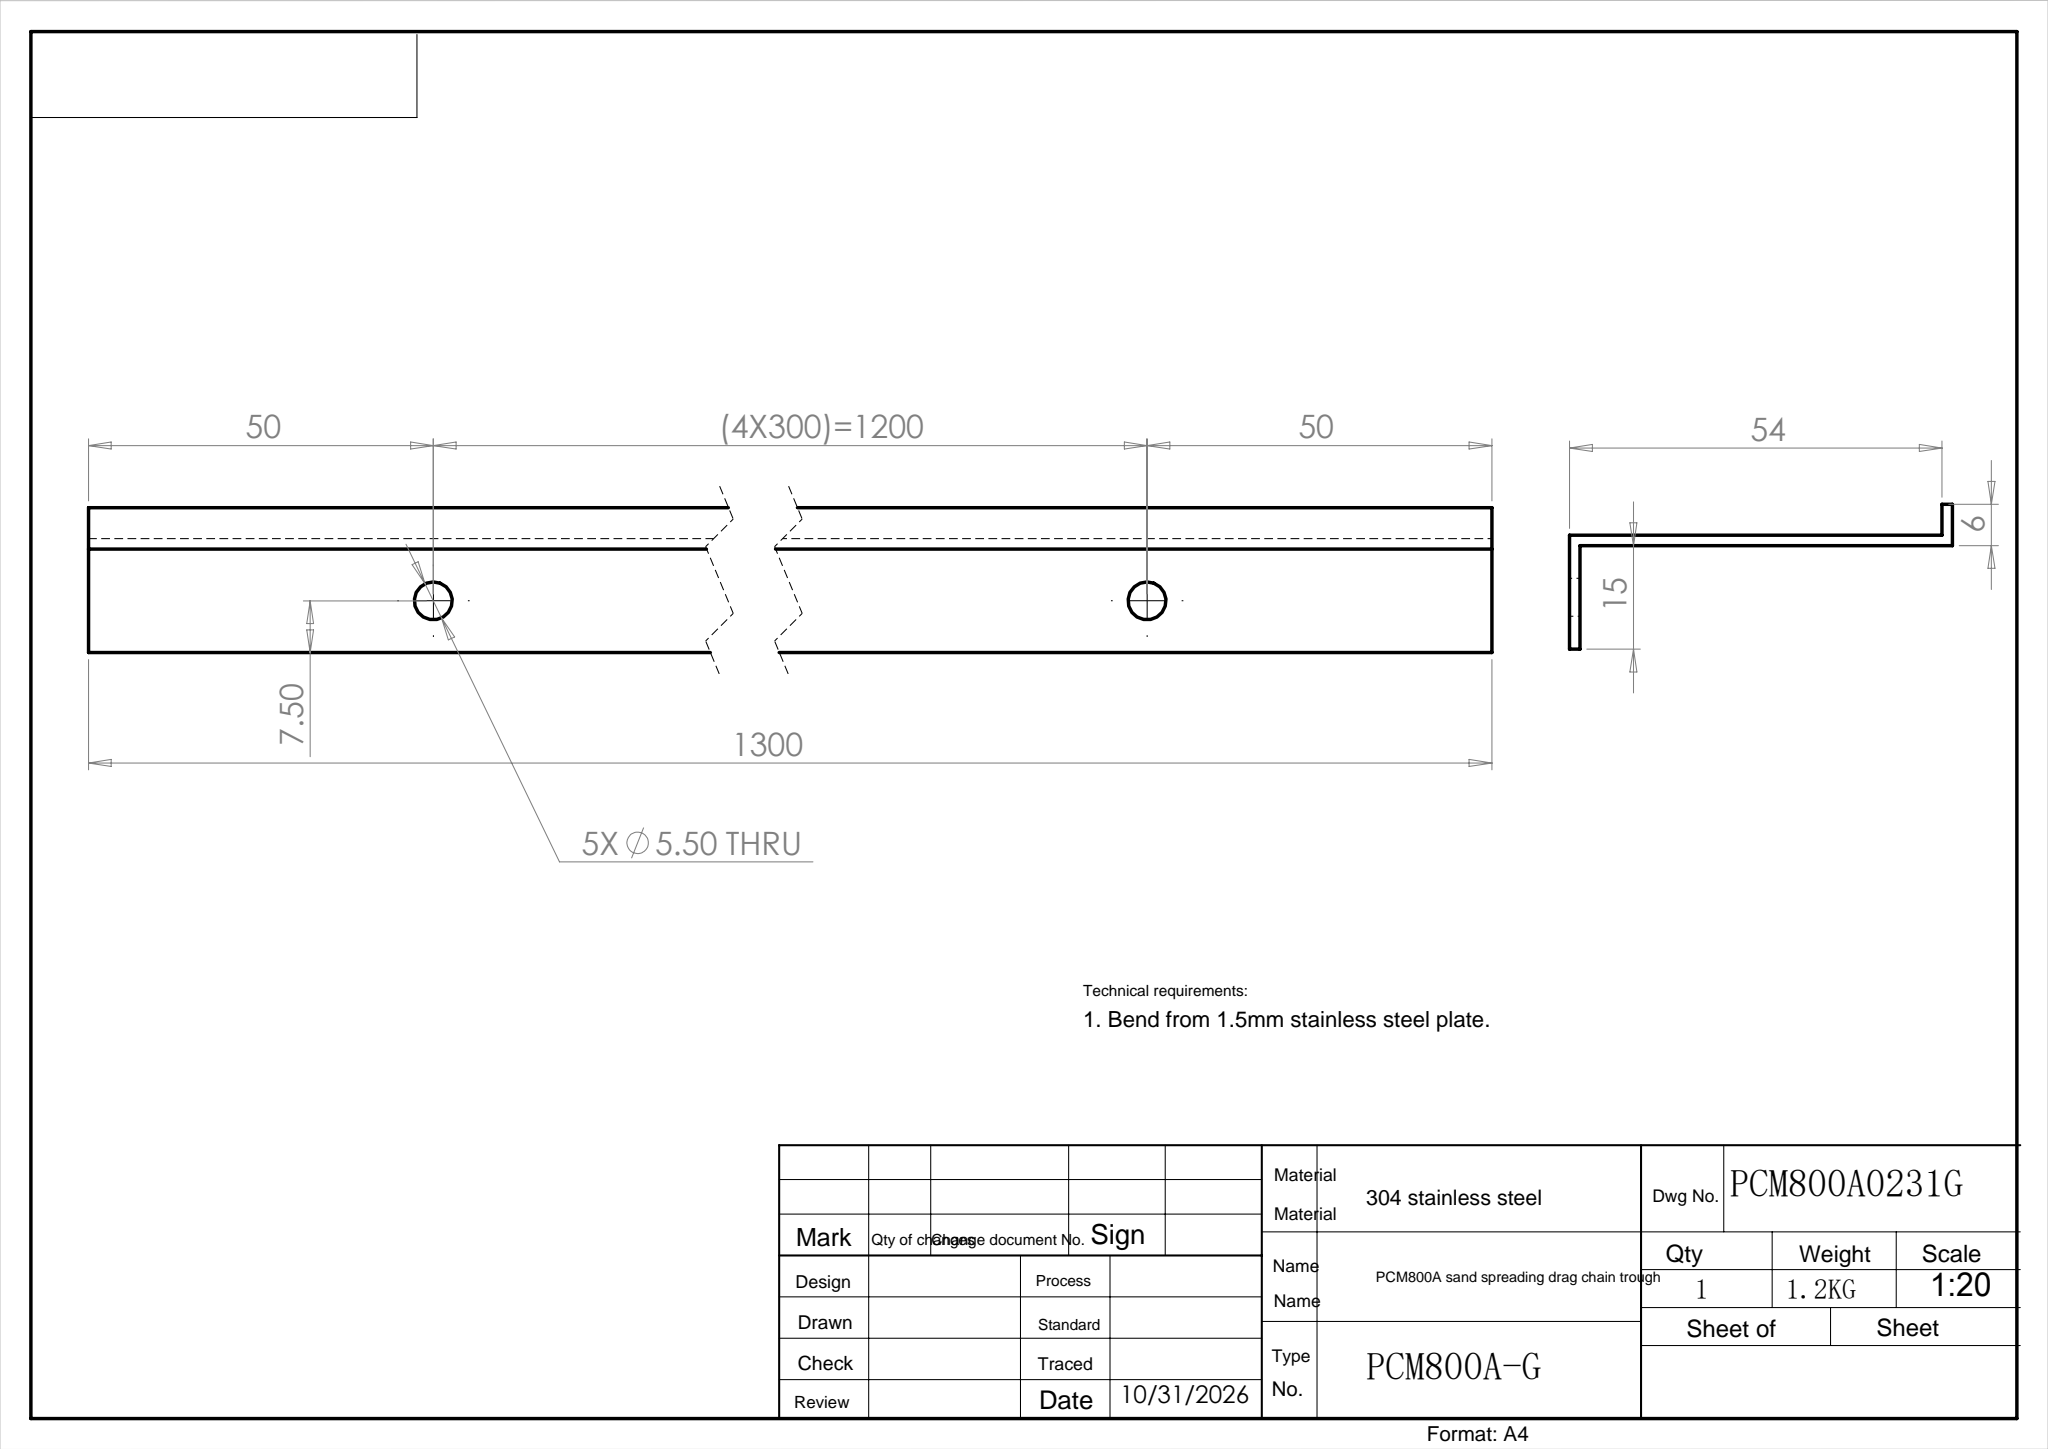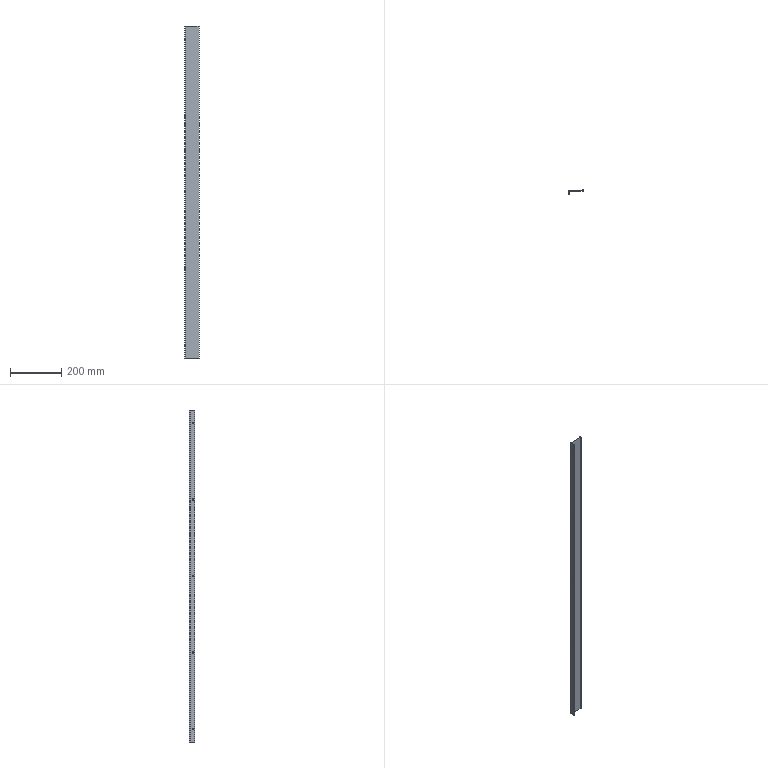Part | SolidWorks | features ExtruThin 1, ICE 1 | 1 solid | 20 faces | box 55.5 x 21 x 1300 mm | volume 146072 mm3 | cylinder 10 | plane 10 | commonest cylinder face diameters 5.5 x10
STEP:
#1=CARTESIAN_POINT('',(-1.5,-4.75,50.));
#2=VERTEX_POINT('',#1);
#3=CARTESIAN_POINT('',(-1.5,-10.25,50.));
#4=VERTEX_POINT('',#3);
#5=CARTESIAN_POINT('',(-1.5,-7.5,50.));
#6=DIRECTION('',(-1.,0.,0.));
#7=DIRECTION('',(0.,-1.,0.));
#8=AXIS2_PLACEMENT_3D('',#5,#6,#7);
#9=CIRCLE('',#8,2.75);
#10=EDGE_CURVE('',#2,#4,#9,.T.);
#11=ORIENTED_EDGE('',*,*,#10,.T.);
#12=CARTESIAN_POINT('',(0.,-10.25,50.));
#13=VERTEX_POINT('',#12);
#14=CARTESIAN_POINT('',(-10.,-10.25,50.));
#15=DIRECTION('',(1.,0.,0.));
#16=VECTOR('',#15,1000.);
#17=LINE('',#14,#16);
#18=EDGE_CURVE('',#4,#13,#17,.T.);
#19=ORIENTED_EDGE('',*,*,#18,.T.);
#20=CARTESIAN_POINT('',(0.,-4.75,50.));
#21=VERTEX_POINT('',#20);
#22=CARTESIAN_POINT('',(0.,-7.5,50.));
#23=DIRECTION('',(1.,0.,0.));
#24=DIRECTION('',(0.,1.,0.));
#25=AXIS2_PLACEMENT_3D('',#22,#23,#24);
#26=CIRCLE('',#25,2.75);
#27=EDGE_CURVE('',#13,#21,#26,.T.);
#28=ORIENTED_EDGE('',*,*,#27,.T.);
#29=CARTESIAN_POINT('',(-10.,-4.75,50.));
#30=DIRECTION('',(1.,0.,0.));
#31=VECTOR('',#30,1000.);
#32=LINE('',#29,#31);
#33=EDGE_CURVE('',#2,#21,#32,.T.);
#34=ORIENTED_EDGE('',*,*,#33,.F.);
#35=EDGE_LOOP('',(#11,#19,#28,#34));
#36=FACE_OUTER_BOUND('',#35,.T.);
#37=CARTESIAN_POINT('',(-10.,-7.5,50.));
#38=DIRECTION('',(1.,0.,0.));
#39=DIRECTION('',(0.,1.,0.));
#40=AXIS2_PLACEMENT_3D('',#37,#38,#39);
#41=CYLINDRICAL_SURFACE('',#40,2.75);
#42=ADVANCED_FACE('',(#36),#41,.F.);
#43=CARTESIAN_POINT('',(-1.5,-4.75,350.));
#44=VERTEX_POINT('',#43);
#45=CARTESIAN_POINT('',(-1.5,-10.25,350.));
#46=VERTEX_POINT('',#45);
#47=CARTESIAN_POINT('',(-1.5,-7.5,350.));
#48=DIRECTION('',(-1.,0.,0.));
#49=DIRECTION('',(0.,-1.,0.));
#50=AXIS2_PLACEMENT_3D('',#47,#48,#49);
#51=CIRCLE('',#50,2.75);
#52=EDGE_CURVE('',#44,#46,#51,.T.);
#53=ORIENTED_EDGE('',*,*,#52,.T.);
#54=CARTESIAN_POINT('',(0.,-10.25,350.));
#55=VERTEX_POINT('',#54);
#56=CARTESIAN_POINT('',(-10.,-10.25,350.));
#57=DIRECTION('',(1.,0.,0.));
#58=VECTOR('',#57,1000.);
#59=LINE('',#56,#58);
#60=EDGE_CURVE('',#46,#55,#59,.T.);
#61=ORIENTED_EDGE('',*,*,#60,.T.);
#62=CARTESIAN_POINT('',(0.,-4.75,350.));
#63=VERTEX_POINT('',#62);
#64=CARTESIAN_POINT('',(0.,-7.5,350.));
#65=DIRECTION('',(1.,0.,0.));
#66=DIRECTION('',(0.,1.,0.));
#67=AXIS2_PLACEMENT_3D('',#64,#65,#66);
#68=CIRCLE('',#67,2.75);
#69=EDGE_CURVE('',#55,#63,#68,.T.);
#70=ORIENTED_EDGE('',*,*,#69,.T.);
#71=CARTESIAN_POINT('',(-10.,-4.75,350.));
#72=DIRECTION('',(1.,0.,0.));
#73=VECTOR('',#72,1000.);
#74=LINE('',#71,#73);
#75=EDGE_CURVE('',#44,#63,#74,.T.);
#76=ORIENTED_EDGE('',*,*,#75,.F.);
#77=EDGE_LOOP('',(#53,#61,#70,#76));
#78=FACE_OUTER_BOUND('',#77,.T.);
#79=CARTESIAN_POINT('',(-10.,-7.5,350.));
#80=DIRECTION('',(1.,0.,0.));
#81=DIRECTION('',(0.,1.,0.));
#82=AXIS2_PLACEMENT_3D('',#79,#80,#81);
#83=CYLINDRICAL_SURFACE('',#82,2.75);
#84=ADVANCED_FACE('',(#78),#83,.F.);
#85=CARTESIAN_POINT('',(-1.5,-4.75,650.));
#86=VERTEX_POINT('',#85);
#87=CARTESIAN_POINT('',(-1.5,-10.25,650.));
#88=VERTEX_POINT('',#87);
#89=CARTESIAN_POINT('',(-1.5,-7.5,650.));
#90=DIRECTION('',(-1.,0.,0.));
#91=DIRECTION('',(0.,-1.,0.));
#92=AXIS2_PLACEMENT_3D('',#89,#90,#91);
#93=CIRCLE('',#92,2.75);
#94=EDGE_CURVE('',#86,#88,#93,.T.);
#95=ORIENTED_EDGE('',*,*,#94,.T.);
#96=CARTESIAN_POINT('',(0.,-10.25,650.));
#97=VERTEX_POINT('',#96);
#98=CARTESIAN_POINT('',(-10.,-10.25,650.));
#99=DIRECTION('',(1.,0.,0.));
#100=VECTOR('',#99,1000.);
#101=LINE('',#98,#100);
#102=EDGE_CURVE('',#88,#97,#101,.T.);
#103=ORIENTED_EDGE('',*,*,#102,.T.);
#104=CARTESIAN_POINT('',(0.,-4.75,650.));
#105=VERTEX_POINT('',#104);
#106=CARTESIAN_POINT('',(0.,-7.5,650.));
#107=DIRECTION('',(1.,0.,0.));
#108=DIRECTION('',(0.,1.,0.));
#109=AXIS2_PLACEMENT_3D('',#106,#107,#108);
#110=CIRCLE('',#109,2.75);
#111=EDGE_CURVE('',#97,#105,#110,.T.);
#112=ORIENTED_EDGE('',*,*,#111,.T.);
#113=CARTESIAN_POINT('',(-10.,-4.75,650.));
#114=DIRECTION('',(1.,0.,0.));
#115=VECTOR('',#114,1000.);
#116=LINE('',#113,#115);
#117=EDGE_CURVE('',#86,#105,#116,.T.);
#118=ORIENTED_EDGE('',*,*,#117,.F.);
#119=EDGE_LOOP('',(#95,#103,#112,#118));
#120=FACE_OUTER_BOUND('',#119,.T.);
#121=CARTESIAN_POINT('',(-10.,-7.5,650.));
#122=DIRECTION('',(1.,0.,0.));
#123=DIRECTION('',(0.,1.,0.));
#124=AXIS2_PLACEMENT_3D('',#121,#122,#123);
#125=CYLINDRICAL_SURFACE('',#124,2.75);
#126=ADVANCED_FACE('',(#120),#125,.F.);
#127=CARTESIAN_POINT('',(-1.5,-4.75,950.));
#128=VERTEX_POINT('',#127);
#129=CARTESIAN_POINT('',(-1.5,-10.25,950.));
#130=VERTEX_POINT('',#129);
#131=CARTESIAN_POINT('',(-1.5,-7.5,950.));
#132=DIRECTION('',(-1.,0.,0.));
#133=DIRECTION('',(0.,-1.,0.));
#134=AXIS2_PLACEMENT_3D('',#131,#132,#133);
#135=CIRCLE('',#134,2.75);
#136=EDGE_CURVE('',#128,#130,#135,.T.);
#137=ORIENTED_EDGE('',*,*,#136,.T.);
#138=CARTESIAN_POINT('',(0.,-10.25,950.));
#139=VERTEX_POINT('',#138);
#140=CARTESIAN_POINT('',(-10.,-10.25,950.));
#141=DIRECTION('',(1.,0.,0.));
#142=VECTOR('',#141,1000.);
#143=LINE('',#140,#142);
#144=EDGE_CURVE('',#130,#139,#143,.T.);
#145=ORIENTED_EDGE('',*,*,#144,.T.);
#146=CARTESIAN_POINT('',(0.,-4.75,950.));
#147=VERTEX_POINT('',#146);
#148=CARTESIAN_POINT('',(0.,-7.5,950.));
#149=DIRECTION('',(1.,0.,0.));
#150=DIRECTION('',(0.,1.,0.));
#151=AXIS2_PLACEMENT_3D('',#148,#149,#150);
#152=CIRCLE('',#151,2.75);
#153=EDGE_CURVE('',#139,#147,#152,.T.);
#154=ORIENTED_EDGE('',*,*,#153,.T.);
#155=CARTESIAN_POINT('',(-10.,-4.75,950.));
#156=DIRECTION('',(1.,0.,0.));
#157=VECTOR('',#156,1000.);
#158=LINE('',#155,#157);
#159=EDGE_CURVE('',#128,#147,#158,.T.);
#160=ORIENTED_EDGE('',*,*,#159,.F.);
#161=EDGE_LOOP('',(#137,#145,#154,#160));
#162=FACE_OUTER_BOUND('',#161,.T.);
#163=CARTESIAN_POINT('',(-10.,-7.5,950.));
#164=DIRECTION('',(1.,0.,0.));
#165=DIRECTION('',(0.,1.,0.));
#166=AXIS2_PLACEMENT_3D('',#163,#164,#165);
#167=CYLINDRICAL_SURFACE('',#166,2.75);
#168=ADVANCED_FACE('',(#162),#167,.F.);
#169=CARTESIAN_POINT('',(-1.5,-4.75,1250.));
#170=VERTEX_POINT('',#169);
#171=CARTESIAN_POINT('',(-1.5,-10.25,1250.));
#172=VERTEX_POINT('',#171);
#173=CARTESIAN_POINT('',(-1.5,-7.5,1250.));
#174=DIRECTION('',(-1.,0.,0.));
#175=DIRECTION('',(0.,-1.,0.));
#176=AXIS2_PLACEMENT_3D('',#173,#174,#175);
#177=CIRCLE('',#176,2.75);
#178=EDGE_CURVE('',#170,#172,#177,.T.);
#179=ORIENTED_EDGE('',*,*,#178,.T.);
#180=CARTESIAN_POINT('',(0.,-10.25,1250.));
#181=VERTEX_POINT('',#180);
#182=CARTESIAN_POINT('',(-10.,-10.25,1250.));
#183=DIRECTION('',(1.,0.,0.));
#184=VECTOR('',#183,1000.);
#185=LINE('',#182,#184);
#186=EDGE_CURVE('',#172,#181,#185,.T.);
#187=ORIENTED_EDGE('',*,*,#186,.T.);
#188=CARTESIAN_POINT('',(0.,-4.75,1250.));
#189=VERTEX_POINT('',#188);
#190=CARTESIAN_POINT('',(0.,-7.5,1250.));
#191=DIRECTION('',(1.,0.,0.));
#192=DIRECTION('',(0.,1.,0.));
#193=AXIS2_PLACEMENT_3D('',#190,#191,#192);
#194=CIRCLE('',#193,2.75);
#195=EDGE_CURVE('',#181,#189,#194,.T.);
#196=ORIENTED_EDGE('',*,*,#195,.T.);
#197=CARTESIAN_POINT('',(-10.,-4.75,1250.));
#198=DIRECTION('',(1.,0.,0.));
#199=VECTOR('',#198,1000.);
#200=LINE('',#197,#199);
#201=EDGE_CURVE('',#170,#189,#200,.T.);
#202=ORIENTED_EDGE('',*,*,#201,.F.);
#203=EDGE_LOOP('',(#179,#187,#196,#202));
#204=FACE_OUTER_BOUND('',#203,.T.);
#205=CARTESIAN_POINT('',(-10.,-7.5,1250.));
#206=DIRECTION('',(1.,0.,0.));
#207=DIRECTION('',(0.,1.,0.));
#208=AXIS2_PLACEMENT_3D('',#205,#206,#207);
#209=CYLINDRICAL_SURFACE('',#208,2.75);
#210=ADVANCED_FACE('',(#204),#209,.F.);
#211=CARTESIAN_POINT('',(54.,0.,0.));
#212=VERTEX_POINT('',#211);
#213=CARTESIAN_POINT('',(54.,6.,0.));
#214=VERTEX_POINT('',#213);
#215=CARTESIAN_POINT('',(54.,0.,0.));
#216=DIRECTION('',(0.,1.,0.));
#217=VECTOR('',#216,1000.);
#218=LINE('',#215,#217);
#219=EDGE_CURVE('',#212,#214,#218,.T.);
#220=ORIENTED_EDGE('',*,*,#219,.T.);
#221=CARTESIAN_POINT('',(54.,6.,1300.));
#222=VERTEX_POINT('',#221);
#223=CARTESIAN_POINT('',(54.,6.,1300.));
#224=DIRECTION('',(0.,0.,-1.));
#225=VECTOR('',#224,1000.);
#226=LINE('',#223,#225);
#227=EDGE_CURVE('',#222,#214,#226,.T.);
#228=ORIENTED_EDGE('',*,*,#227,.F.);
#229=CARTESIAN_POINT('',(54.,0.,1300.));
#230=VERTEX_POINT('',#229);
#231=CARTESIAN_POINT('',(54.,0.,1300.));
#232=DIRECTION('',(0.,1.,0.));
#233=VECTOR('',#232,1000.);
#234=LINE('',#231,#233);
#235=EDGE_CURVE('',#230,#222,#234,.T.);
#236=ORIENTED_EDGE('',*,*,#235,.F.);
#237=CARTESIAN_POINT('',(54.,0.,1300.));
#238=DIRECTION('',(0.,0.,-1.));
#239=VECTOR('',#238,1000.);
#240=LINE('',#237,#239);
#241=EDGE_CURVE('',#230,#212,#240,.T.);
#242=ORIENTED_EDGE('',*,*,#241,.T.);
#243=EDGE_LOOP('',(#220,#228,#236,#242));
#244=FACE_OUTER_BOUND('',#243,.T.);
#245=CARTESIAN_POINT('',(54.,0.,1300.));
#246=DIRECTION('',(-1.,0.,0.));
#247=DIRECTION('',(0.,0.,1.));
#248=AXIS2_PLACEMENT_3D('',#245,#246,#247);
#249=PLANE('',#248);
#250=ADVANCED_FACE('',(#244),#249,.F.);
#251=CARTESIAN_POINT('',(52.5,6.,0.));
#252=VERTEX_POINT('',#251);
#253=CARTESIAN_POINT('',(52.5,6.,0.));
#254=DIRECTION('',(1.,0.,0.));
#255=VECTOR('',#254,1000.);
#256=LINE('',#253,#255);
#257=EDGE_CURVE('',#252,#214,#256,.T.);
#258=ORIENTED_EDGE('',*,*,#257,.F.);
#259=CARTESIAN_POINT('',(52.5,6.,1300.));
#260=VERTEX_POINT('',#259);
#261=CARTESIAN_POINT('',(52.5,6.,1300.));
#262=DIRECTION('',(0.,0.,-1.));
#263=VECTOR('',#262,1000.);
#264=LINE('',#261,#263);
#265=EDGE_CURVE('',#260,#252,#264,.T.);
#266=ORIENTED_EDGE('',*,*,#265,.F.);
#267=CARTESIAN_POINT('',(52.5,6.,1300.));
#268=DIRECTION('',(1.,0.,0.));
#269=VECTOR('',#268,1000.);
#270=LINE('',#267,#269);
#271=EDGE_CURVE('',#260,#222,#270,.T.);
#272=ORIENTED_EDGE('',*,*,#271,.T.);
#273=ORIENTED_EDGE('',*,*,#227,.T.);
#274=EDGE_LOOP('',(#258,#266,#272,#273));
#275=FACE_OUTER_BOUND('',#274,.T.);
#276=CARTESIAN_POINT('',(52.5,6.,1300.));
#277=DIRECTION('',(0.,1.,0.));
#278=DIRECTION('',(0.,0.,1.));
#279=AXIS2_PLACEMENT_3D('',#276,#277,#278);
#280=PLANE('',#279);
#281=ADVANCED_FACE('',(#275),#280,.T.);
#282=CARTESIAN_POINT('',(52.5,1.5,0.));
#283=VERTEX_POINT('',#282);
#284=CARTESIAN_POINT('',(52.5,0.,0.));
#285=DIRECTION('',(0.,1.,0.));
#286=VECTOR('',#285,1000.);
#287=LINE('',#284,#286);
#288=EDGE_CURVE('',#283,#252,#287,.T.);
#289=ORIENTED_EDGE('',*,*,#288,.F.);
#290=CARTESIAN_POINT('',(52.5,1.5,1300.));
#291=VERTEX_POINT('',#290);
#292=CARTESIAN_POINT('',(52.5,1.5,1300.));
#293=DIRECTION('',(0.,0.,-1.));
#294=VECTOR('',#293,1000.);
#295=LINE('',#292,#294);
#296=EDGE_CURVE('',#291,#283,#295,.T.);
#297=ORIENTED_EDGE('',*,*,#296,.F.);
#298=CARTESIAN_POINT('',(52.5,0.,1300.));
#299=DIRECTION('',(0.,1.,0.));
#300=VECTOR('',#299,1000.);
#301=LINE('',#298,#300);
#302=EDGE_CURVE('',#291,#260,#301,.T.);
#303=ORIENTED_EDGE('',*,*,#302,.T.);
#304=ORIENTED_EDGE('',*,*,#265,.T.);
#305=EDGE_LOOP('',(#289,#297,#303,#304));
#306=FACE_OUTER_BOUND('',#305,.T.);
#307=CARTESIAN_POINT('',(52.5,0.,1300.));
#308=DIRECTION('',(-1.,0.,0.));
#309=DIRECTION('',(0.,0.,1.));
#310=AXIS2_PLACEMENT_3D('',#307,#308,#309);
#311=PLANE('',#310);
#312=ADVANCED_FACE('',(#306),#311,.T.);
#313=CARTESIAN_POINT('',(-1.5,1.5,0.));
#314=VERTEX_POINT('',#313);
#315=CARTESIAN_POINT('',(0.,1.5,0.));
#316=DIRECTION('',(1.,0.,0.));
#317=VECTOR('',#316,1000.);
#318=LINE('',#315,#317);
#319=EDGE_CURVE('',#314,#283,#318,.T.);
#320=ORIENTED_EDGE('',*,*,#319,.F.);
#321=CARTESIAN_POINT('',(-1.5,1.5,1300.));
#322=VERTEX_POINT('',#321);
#323=CARTESIAN_POINT('',(-1.5,1.5,1300.));
#324=DIRECTION('',(0.,0.,-1.));
#325=VECTOR('',#324,1000.);
#326=LINE('',#323,#325);
#327=EDGE_CURVE('',#322,#314,#326,.T.);
#328=ORIENTED_EDGE('',*,*,#327,.F.);
#329=CARTESIAN_POINT('',(0.,1.5,1300.));
#330=DIRECTION('',(1.,0.,0.));
#331=VECTOR('',#330,1000.);
#332=LINE('',#329,#331);
#333=EDGE_CURVE('',#322,#291,#332,.T.);
#334=ORIENTED_EDGE('',*,*,#333,.T.);
#335=ORIENTED_EDGE('',*,*,#296,.T.);
#336=EDGE_LOOP('',(#320,#328,#334,#335));
#337=FACE_OUTER_BOUND('',#336,.T.);
#338=CARTESIAN_POINT('',(0.,1.5,1300.));
#339=DIRECTION('',(0.,1.,0.));
#340=DIRECTION('',(0.,0.,1.));
#341=AXIS2_PLACEMENT_3D('',#338,#339,#340);
#342=PLANE('',#341);
#343=ADVANCED_FACE('',(#337),#342,.T.);
#344=ORIENTED_EDGE('',*,*,#10,.F.);
#345=CARTESIAN_POINT('',(-1.5,-7.5,50.));
#346=DIRECTION('',(-1.,0.,0.));
#347=DIRECTION('',(0.,-1.,0.));
#348=AXIS2_PLACEMENT_3D('',#345,#346,#347);
#349=CIRCLE('',#348,2.75);
#350=EDGE_CURVE('',#4,#2,#349,.T.);
#351=ORIENTED_EDGE('',*,*,#350,.F.);
#352=EDGE_LOOP('',(#344,#351));
#353=FACE_BOUND('',#352,.T.);
#354=ORIENTED_EDGE('',*,*,#52,.F.);
#355=CARTESIAN_POINT('',(-1.5,-7.5,350.));
#356=DIRECTION('',(-1.,0.,0.));
#357=DIRECTION('',(0.,-1.,0.));
#358=AXIS2_PLACEMENT_3D('',#355,#356,#357);
#359=CIRCLE('',#358,2.75);
#360=EDGE_CURVE('',#46,#44,#359,.T.);
#361=ORIENTED_EDGE('',*,*,#360,.F.);
#362=EDGE_LOOP('',(#354,#361));
#363=FACE_BOUND('',#362,.T.);
#364=ORIENTED_EDGE('',*,*,#94,.F.);
#365=CARTESIAN_POINT('',(-1.5,-7.5,650.));
#366=DIRECTION('',(-1.,0.,0.));
#367=DIRECTION('',(0.,-1.,0.));
#368=AXIS2_PLACEMENT_3D('',#365,#366,#367);
#369=CIRCLE('',#368,2.75);
#370=EDGE_CURVE('',#88,#86,#369,.T.);
#371=ORIENTED_EDGE('',*,*,#370,.F.);
#372=EDGE_LOOP('',(#364,#371));
#373=FACE_BOUND('',#372,.T.);
#374=ORIENTED_EDGE('',*,*,#136,.F.);
#375=CARTESIAN_POINT('',(-1.5,-7.5,950.));
#376=DIRECTION('',(-1.,0.,0.));
#377=DIRECTION('',(0.,-1.,0.));
#378=AXIS2_PLACEMENT_3D('',#375,#376,#377);
#379=CIRCLE('',#378,2.75);
#380=EDGE_CURVE('',#130,#128,#379,.T.);
#381=ORIENTED_EDGE('',*,*,#380,.F.);
#382=EDGE_LOOP('',(#374,#381));
#383=FACE_BOUND('',#382,.T.);
#384=ORIENTED_EDGE('',*,*,#178,.F.);
#385=CARTESIAN_POINT('',(-1.5,-7.5,1250.));
#386=DIRECTION('',(-1.,0.,0.));
#387=DIRECTION('',(0.,-1.,0.));
#388=AXIS2_PLACEMENT_3D('',#385,#386,#387);
#389=CIRCLE('',#388,2.75);
#390=EDGE_CURVE('',#172,#170,#389,.T.);
#391=ORIENTED_EDGE('',*,*,#390,.F.);
#392=EDGE_LOOP('',(#384,#391));
#393=FACE_BOUND('',#392,.T.);
#394=CARTESIAN_POINT('',(-1.5,-15.,0.));
#395=VERTEX_POINT('',#394);
#396=CARTESIAN_POINT('',(-1.5,0.,0.));
#397=DIRECTION('',(0.,1.,0.));
#398=VECTOR('',#397,1000.);
#399=LINE('',#396,#398);
#400=EDGE_CURVE('',#395,#314,#399,.T.);
#401=ORIENTED_EDGE('',*,*,#400,.F.);
#402=CARTESIAN_POINT('',(-1.5,-15.,1300.));
#403=VERTEX_POINT('',#402);
#404=CARTESIAN_POINT('',(-1.5,-15.,1300.));
#405=DIRECTION('',(0.,0.,-1.));
#406=VECTOR('',#405,1000.);
#407=LINE('',#404,#406);
#408=EDGE_CURVE('',#403,#395,#407,.T.);
#409=ORIENTED_EDGE('',*,*,#408,.F.);
#410=CARTESIAN_POINT('',(-1.5,0.,1300.));
#411=DIRECTION('',(0.,1.,0.));
#412=VECTOR('',#411,1000.);
#413=LINE('',#410,#412);
#414=EDGE_CURVE('',#403,#322,#413,.T.);
#415=ORIENTED_EDGE('',*,*,#414,.T.);
#416=ORIENTED_EDGE('',*,*,#327,.T.);
#417=EDGE_LOOP('',(#401,#409,#415,#416));
#418=FACE_OUTER_BOUND('',#417,.T.);
#419=CARTESIAN_POINT('',(-1.5,0.,1300.));
#420=DIRECTION('',(-1.,0.,0.));
#421=DIRECTION('',(0.,-1.,0.));
#422=AXIS2_PLACEMENT_3D('',#419,#420,#421);
#423=PLANE('',#422);
#424=ADVANCED_FACE('',(#353,#363,#373,#383,#393,#418),#423,.T.);
#425=CARTESIAN_POINT('',(0.,-15.,0.));
#426=VERTEX_POINT('',#425);
#427=CARTESIAN_POINT('',(0.,-15.,0.));
#428=DIRECTION('',(-1.,0.,0.));
#429=VECTOR('',#428,1000.);
#430=LINE('',#427,#429);
#431=EDGE_CURVE('',#426,#395,#430,.T.);
#432=ORIENTED_EDGE('',*,*,#431,.F.);
#433=CARTESIAN_POINT('',(0.,-15.,1300.));
#434=VERTEX_POINT('',#433);
#435=CARTESIAN_POINT('',(0.,-15.,1300.));
#436=DIRECTION('',(0.,0.,-1.));
#437=VECTOR('',#436,1000.);
#438=LINE('',#435,#437);
#439=EDGE_CURVE('',#434,#426,#438,.T.);
#440=ORIENTED_EDGE('',*,*,#439,.F.);
#441=CARTESIAN_POINT('',(0.,-15.,1300.));
#442=DIRECTION('',(-1.,0.,0.));
#443=VECTOR('',#442,1000.);
#444=LINE('',#441,#443);
#445=EDGE_CURVE('',#434,#403,#444,.T.);
#446=ORIENTED_EDGE('',*,*,#445,.T.);
#447=ORIENTED_EDGE('',*,*,#408,.T.);
#448=EDGE_LOOP('',(#432,#440,#446,#447));
#449=FACE_OUTER_BOUND('',#448,.T.);
#450=CARTESIAN_POINT('',(0.,-15.,1300.));
#451=DIRECTION('',(0.,-1.,0.));
#452=DIRECTION('',(0.,0.,-1.));
#453=AXIS2_PLACEMENT_3D('',#450,#451,#452);
#454=PLANE('',#453);
#455=ADVANCED_FACE('',(#449),#454,.T.);
#456=CARTESIAN_POINT('',(0.,-7.5,50.));
#457=DIRECTION('',(1.,0.,0.));
#458=DIRECTION('',(0.,1.,0.));
#459=AXIS2_PLACEMENT_3D('',#456,#457,#458);
#460=CIRCLE('',#459,2.75);
#461=EDGE_CURVE('',#21,#13,#460,.T.);
#462=ORIENTED_EDGE('',*,*,#461,.F.);
#463=ORIENTED_EDGE('',*,*,#27,.F.);
#464=EDGE_LOOP('',(#462,#463));
#465=FACE_BOUND('',#464,.T.);
#466=CARTESIAN_POINT('',(0.,-7.5,350.));
#467=DIRECTION('',(1.,0.,0.));
#468=DIRECTION('',(0.,1.,0.));
#469=AXIS2_PLACEMENT_3D('',#466,#467,#468);
#470=CIRCLE('',#469,2.75);
#471=EDGE_CURVE('',#63,#55,#470,.T.);
#472=ORIENTED_EDGE('',*,*,#471,.F.);
#473=ORIENTED_EDGE('',*,*,#69,.F.);
#474=EDGE_LOOP('',(#472,#473));
#475=FACE_BOUND('',#474,.T.);
#476=CARTESIAN_POINT('',(0.,-7.5,650.));
#477=DIRECTION('',(1.,0.,0.));
#478=DIRECTION('',(0.,1.,0.));
#479=AXIS2_PLACEMENT_3D('',#476,#477,#478);
#480=CIRCLE('',#479,2.75);
#481=EDGE_CURVE('',#105,#97,#480,.T.);
#482=ORIENTED_EDGE('',*,*,#481,.F.);
#483=ORIENTED_EDGE('',*,*,#111,.F.);
#484=EDGE_LOOP('',(#482,#483));
#485=FACE_BOUND('',#484,.T.);
#486=CARTESIAN_POINT('',(0.,-7.5,950.));
#487=DIRECTION('',(1.,0.,0.));
#488=DIRECTION('',(0.,1.,0.));
#489=AXIS2_PLACEMENT_3D('',#486,#487,#488);
#490=CIRCLE('',#489,2.75);
#491=EDGE_CURVE('',#147,#139,#490,.T.);
#492=ORIENTED_EDGE('',*,*,#491,.F.);
#493=ORIENTED_EDGE('',*,*,#153,.F.);
#494=EDGE_LOOP('',(#492,#493));
#495=FACE_BOUND('',#494,.T.);
#496=CARTESIAN_POINT('',(0.,-7.5,1250.));
#497=DIRECTION('',(1.,0.,0.));
#498=DIRECTION('',(0.,1.,0.));
#499=AXIS2_PLACEMENT_3D('',#496,#497,#498);
#500=CIRCLE('',#499,2.75);
#501=EDGE_CURVE('',#189,#181,#500,.T.);
#502=ORIENTED_EDGE('',*,*,#501,.F.);
#503=ORIENTED_EDGE('',*,*,#195,.F.);
#504=EDGE_LOOP('',(#502,#503));
#505=FACE_BOUND('',#504,.T.);
#506=CARTESIAN_POINT('',(0.,0.,0.));
#507=VERTEX_POINT('',#506);
#508=CARTESIAN_POINT('',(0.,0.,0.));
#509=DIRECTION('',(0.,1.,0.));
#510=VECTOR('',#509,1000.);
#511=LINE('',#508,#510);
#512=EDGE_CURVE('',#426,#507,#511,.T.);
#513=ORIENTED_EDGE('',*,*,#512,.T.);
#514=CARTESIAN_POINT('',(0.,0.,1300.));
#515=VERTEX_POINT('',#514);
#516=CARTESIAN_POINT('',(0.,0.,1300.));
#517=DIRECTION('',(0.,0.,-1.));
#518=VECTOR('',#517,1000.);
#519=LINE('',#516,#518);
#520=EDGE_CURVE('',#515,#507,#519,.T.);
#521=ORIENTED_EDGE('',*,*,#520,.F.);
#522=CARTESIAN_POINT('',(0.,0.,1300.));
#523=DIRECTION('',(0.,1.,0.));
#524=VECTOR('',#523,1000.);
#525=LINE('',#522,#524);
#526=EDGE_CURVE('',#434,#515,#525,.T.);
#527=ORIENTED_EDGE('',*,*,#526,.F.);
#528=ORIENTED_EDGE('',*,*,#439,.T.);
#529=EDGE_LOOP('',(#513,#521,#527,#528));
#530=FACE_OUTER_BOUND('',#529,.T.);
#531=CARTESIAN_POINT('',(0.,0.,1300.));
#532=DIRECTION('',(-1.,0.,0.));
#533=DIRECTION('',(0.,-1.,0.));
#534=AXIS2_PLACEMENT_3D('',#531,#532,#533);
#535=PLANE('',#534);
#536=ADVANCED_FACE('',(#465,#475,#485,#495,#505,#530),#535,.F.);
#537=CARTESIAN_POINT('',(0.,0.,0.));
#538=DIRECTION('',(1.,0.,0.));
#539=VECTOR('',#538,1000.);
#540=LINE('',#537,#539);
#541=EDGE_CURVE('',#507,#212,#540,.T.);
#542=ORIENTED_EDGE('',*,*,#541,.T.);
#543=ORIENTED_EDGE('',*,*,#241,.F.);
#544=CARTESIAN_POINT('',(0.,0.,1300.));
#545=DIRECTION('',(1.,0.,0.));
#546=VECTOR('',#545,1000.);
#547=LINE('',#544,#546);
#548=EDGE_CURVE('',#515,#230,#547,.T.);
#549=ORIENTED_EDGE('',*,*,#548,.F.);
#550=ORIENTED_EDGE('',*,*,#520,.T.);
#551=EDGE_LOOP('',(#542,#543,#549,#550));
#552=FACE_OUTER_BOUND('',#551,.T.);
#553=CARTESIAN_POINT('',(0.,0.,1300.));
#554=DIRECTION('',(0.,1.,0.));
#555=DIRECTION('',(0.,0.,1.));
#556=AXIS2_PLACEMENT_3D('',#553,#554,#555);
#557=PLANE('',#556);
#558=ADVANCED_FACE('',(#552),#557,.F.);
#559=ORIENTED_EDGE('',*,*,#235,.T.);
#560=ORIENTED_EDGE('',*,*,#271,.F.);
#561=ORIENTED_EDGE('',*,*,#302,.F.);
#562=ORIENTED_EDGE('',*,*,#333,.F.);
#563=ORIENTED_EDGE('',*,*,#414,.F.);
#564=ORIENTED_EDGE('',*,*,#445,.F.);
#565=ORIENTED_EDGE('',*,*,#526,.T.);
#566=ORIENTED_EDGE('',*,*,#548,.T.);
#567=EDGE_LOOP('',(#559,#560,#561,#562,#563,#564,#565,#566));
#568=FACE_OUTER_BOUND('',#567,.T.);
#569=CARTESIAN_POINT('',(54.,6.,1300.));
#570=DIRECTION('',(0.,0.,-1.));
#571=DIRECTION('',(-1.,0.,0.));
#572=AXIS2_PLACEMENT_3D('',#569,#570,#571);
#573=PLANE('',#572);
#574=ADVANCED_FACE('',(#568),#573,.F.);
#575=ORIENTED_EDGE('',*,*,#219,.F.);
#576=ORIENTED_EDGE('',*,*,#541,.F.);
#577=ORIENTED_EDGE('',*,*,#512,.F.);
#578=ORIENTED_EDGE('',*,*,#431,.T.);
#579=ORIENTED_EDGE('',*,*,#400,.T.);
#580=ORIENTED_EDGE('',*,*,#319,.T.);
#581=ORIENTED_EDGE('',*,*,#288,.T.);
#582=ORIENTED_EDGE('',*,*,#257,.T.);
#583=EDGE_LOOP('',(#575,#576,#577,#578,#579,#580,#581,#582));
#584=FACE_OUTER_BOUND('',#583,.T.);
#585=CARTESIAN_POINT('',(54.,6.,0.));
#586=DIRECTION('',(0.,0.,-1.));
#587=DIRECTION('',(-1.,0.,0.));
#588=AXIS2_PLACEMENT_3D('',#585,#586,#587);
#589=PLANE('',#588);
#590=ADVANCED_FACE('',(#584),#589,.T.);
#591=ORIENTED_EDGE('',*,*,#186,.F.);
#592=ORIENTED_EDGE('',*,*,#390,.T.);
#593=ORIENTED_EDGE('',*,*,#201,.T.);
#594=ORIENTED_EDGE('',*,*,#501,.T.);
#595=EDGE_LOOP('',(#591,#592,#593,#594));
#596=FACE_OUTER_BOUND('',#595,.T.);
#597=CARTESIAN_POINT('',(-10.,-7.5,1250.));
#598=DIRECTION('',(1.,0.,0.));
#599=DIRECTION('',(0.,1.,0.));
#600=AXIS2_PLACEMENT_3D('',#597,#598,#599);
#601=CYLINDRICAL_SURFACE('',#600,2.75);
#602=ADVANCED_FACE('',(#596),#601,.F.);
#603=ORIENTED_EDGE('',*,*,#144,.F.);
#604=ORIENTED_EDGE('',*,*,#380,.T.);
#605=ORIENTED_EDGE('',*,*,#159,.T.);
#606=ORIENTED_EDGE('',*,*,#491,.T.);
#607=EDGE_LOOP('',(#603,#604,#605,#606));
#608=FACE_OUTER_BOUND('',#607,.T.);
#609=CARTESIAN_POINT('',(-10.,-7.5,950.));
#610=DIRECTION('',(1.,0.,0.));
#611=DIRECTION('',(0.,1.,0.));
#612=AXIS2_PLACEMENT_3D('',#609,#610,#611);
#613=CYLINDRICAL_SURFACE('',#612,2.75);
#614=ADVANCED_FACE('',(#608),#613,.F.);
#615=ORIENTED_EDGE('',*,*,#102,.F.);
#616=ORIENTED_EDGE('',*,*,#370,.T.);
#617=ORIENTED_EDGE('',*,*,#117,.T.);
#618=ORIENTED_EDGE('',*,*,#481,.T.);
#619=EDGE_LOOP('',(#615,#616,#617,#618));
#620=FACE_OUTER_BOUND('',#619,.T.);
#621=CARTESIAN_POINT('',(-10.,-7.5,650.));
#622=DIRECTION('',(1.,0.,0.));
#623=DIRECTION('',(0.,1.,0.));
#624=AXIS2_PLACEMENT_3D('',#621,#622,#623);
#625=CYLINDRICAL_SURFACE('',#624,2.75);
#626=ADVANCED_FACE('',(#620),#625,.F.);
#627=ORIENTED_EDGE('',*,*,#60,.F.);
#628=ORIENTED_EDGE('',*,*,#360,.T.);
#629=ORIENTED_EDGE('',*,*,#75,.T.);
#630=ORIENTED_EDGE('',*,*,#471,.T.);
#631=EDGE_LOOP('',(#627,#628,#629,#630));
#632=FACE_OUTER_BOUND('',#631,.T.);
#633=CARTESIAN_POINT('',(-10.,-7.5,350.));
#634=DIRECTION('',(1.,0.,0.));
#635=DIRECTION('',(0.,1.,0.));
#636=AXIS2_PLACEMENT_3D('',#633,#634,#635);
#637=CYLINDRICAL_SURFACE('',#636,2.75);
#638=ADVANCED_FACE('',(#632),#637,.F.);
#639=ORIENTED_EDGE('',*,*,#18,.F.);
#640=ORIENTED_EDGE('',*,*,#350,.T.);
#641=ORIENTED_EDGE('',*,*,#33,.T.);
#642=ORIENTED_EDGE('',*,*,#461,.T.);
#643=EDGE_LOOP('',(#639,#640,#641,#642));
#644=FACE_OUTER_BOUND('',#643,.T.);
#645=CARTESIAN_POINT('',(-10.,-7.5,50.));
#646=DIRECTION('',(1.,0.,0.));
#647=DIRECTION('',(0.,1.,0.));
#648=AXIS2_PLACEMENT_3D('',#645,#646,#647);
#649=CYLINDRICAL_SURFACE('',#648,2.75);
#650=ADVANCED_FACE('',(#644),#649,.F.);
#651=CLOSED_SHELL('',(#42,#84,#126,#168,#210,#250,#281,#312,#343,#424,#455,#536,#558,#574,#590,#602,#614,#626,#638,#650));
#652=MANIFOLD_SOLID_BREP('',#651);
#653=CARTESIAN_POINT('',(0.,0.,0.));
#654=DIRECTION('',(0.,0.,1.));
#655=DIRECTION('',(1.,0.,0.));
#656=AXIS2_PLACEMENT_3D('',#653,#654,#655);
#657=(LENGTH_UNIT()NAMED_UNIT(*)SI_UNIT(.MILLI.,.METRE.));
#658=UNCERTAINTY_MEASURE_WITH_UNIT(LENGTH_MEASURE(0.00001),#657,'','');
#659=(NAMED_UNIT(*)PLANE_ANGLE_UNIT()SI_UNIT($,.RADIAN.));
#660=(NAMED_UNIT(*)SI_UNIT($,.STERADIAN.)SOLID_ANGLE_UNIT());
#661=(GEOMETRIC_REPRESENTATION_CONTEXT(3)GLOBAL_UNCERTAINTY_ASSIGNED_CONTEXT((#658))GLOBAL_UNIT_ASSIGNED_CONTEXT((#657,#659,#660))REPRESENTATION_CONTEXT('',''));
#662=ADVANCED_BREP_SHAPE_REPRESENTATION('',(#652,#656),#661);